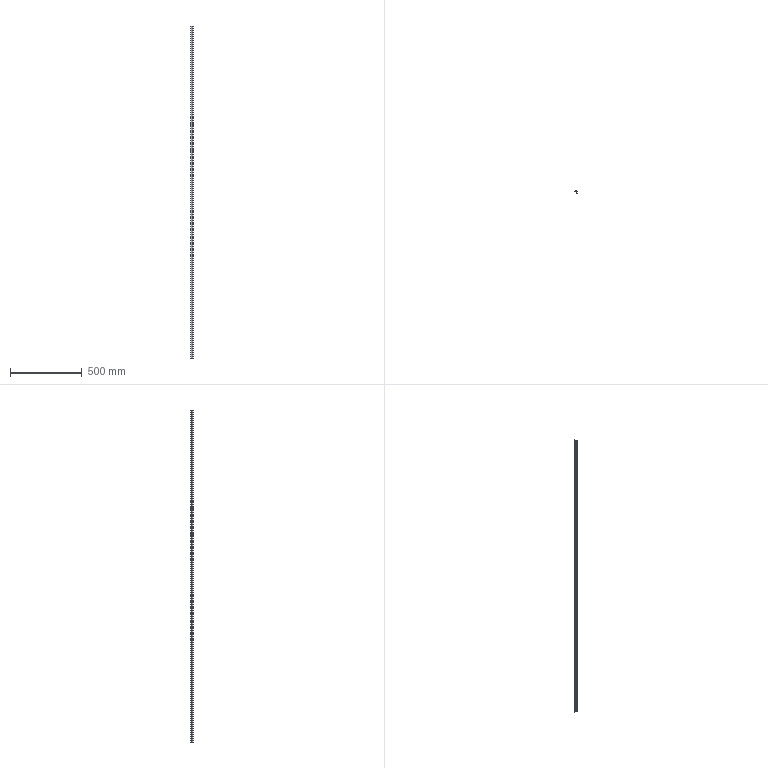Part | SolidWorks | features BaseBody 1, ICE 1, MoveFace 1 | 1 solid | 27 faces | box 14 x 20.3 x 2314 mm | volume 117819 mm3 | plane 20 | cylinder 7 | commonest cylinder face diameters 0.387 x2 0.8 x2 0.4 x1 20 x1 22 x1
STEP:
#1=CARTESIAN_POINT('',(-5.304,-0.625,200.));
#2=VERTEX_POINT('',#1);
#3=CARTESIAN_POINT('',(-5.449,-0.8125,200.));
#4=VERTEX_POINT('',#3);
#5=CARTESIAN_POINT('',(-5.255,-0.8125,200.));
#6=DIRECTION('',(0.,0.,1.));
#7=DIRECTION('',(-1.,0.,0.));
#8=AXIS2_PLACEMENT_3D('',#5,#6,#7);
#9=CIRCLE('',#8,0.1937);
#10=EDGE_CURVE('',#2,#4,#9,.T.);
#11=ORIENTED_EDGE('',*,*,#10,.T.);
#12=CARTESIAN_POINT('',(-5.449,-0.8125,-2114.));
#13=VERTEX_POINT('',#12);
#14=CARTESIAN_POINT('',(-5.449,-0.8125,230.));
#15=DIRECTION('',(0.,0.,-1.));
#16=VECTOR('',#15,1000.);
#17=LINE('',#14,#16);
#18=EDGE_CURVE('',#4,#13,#17,.T.);
#19=ORIENTED_EDGE('',*,*,#18,.T.);
#20=CARTESIAN_POINT('',(-5.304,-0.625,-2114.));
#21=VERTEX_POINT('',#20);
#22=CARTESIAN_POINT('',(-5.255,-0.8125,-2114.));
#23=DIRECTION('',(0.,0.,-1.));
#24=DIRECTION('',(1.,0.,0.));
#25=AXIS2_PLACEMENT_3D('',#22,#23,#24);
#26=CIRCLE('',#25,0.1937);
#27=EDGE_CURVE('',#13,#21,#26,.T.);
#28=ORIENTED_EDGE('',*,*,#27,.T.);
#29=CARTESIAN_POINT('',(-5.304,-0.625,230.));
#30=DIRECTION('',(0.,0.,-1.));
#31=VECTOR('',#30,1000.);
#32=LINE('',#29,#31);
#33=EDGE_CURVE('',#2,#21,#32,.T.);
#34=ORIENTED_EDGE('',*,*,#33,.F.);
#35=EDGE_LOOP('',(#11,#19,#28,#34));
#36=FACE_OUTER_BOUND('',#35,.T.);
#37=CARTESIAN_POINT('',(-5.255,-0.8125,230.));
#38=DIRECTION('',(0.,0.,-1.));
#39=DIRECTION('',(-1.,0.,0.));
#40=AXIS2_PLACEMENT_3D('',#37,#38,#39);
#41=CYLINDRICAL_SURFACE('',#40,0.1937);
#42=ADVANCED_FACE('',(#36),#41,.F.);
#43=CARTESIAN_POINT('',(5.,-1.,-2114.));
#44=VERTEX_POINT('',#43);
#45=CARTESIAN_POINT('',(5.,-14.3,-2114.));
#46=VERTEX_POINT('',#45);
#47=CARTESIAN_POINT('',(5.,29.623,-2114.));
#48=DIRECTION('',(0.,-1.,0.));
#49=VECTOR('',#48,1000.);
#50=LINE('',#47,#49);
#51=EDGE_CURVE('',#44,#46,#50,.T.);
#52=ORIENTED_EDGE('',*,*,#51,.F.);
#53=CARTESIAN_POINT('',(5.,-1.,200.));
#54=VERTEX_POINT('',#53);
#55=CARTESIAN_POINT('',(5.,-1.,230.));
#56=DIRECTION('',(0.,0.,-1.));
#57=VECTOR('',#56,1000.);
#58=LINE('',#55,#57);
#59=EDGE_CURVE('',#54,#44,#58,.T.);
#60=ORIENTED_EDGE('',*,*,#59,.F.);
#61=CARTESIAN_POINT('',(5.,-14.3,200.));
#62=VERTEX_POINT('',#61);
#63=CARTESIAN_POINT('',(5.,-14.3,200.));
#64=DIRECTION('',(0.,1.,0.));
#65=VECTOR('',#64,1000.);
#66=LINE('',#63,#65);
#67=EDGE_CURVE('',#62,#54,#66,.T.);
#68=ORIENTED_EDGE('',*,*,#67,.F.);
#69=CARTESIAN_POINT('',(5.,-14.3,230.));
#70=DIRECTION('',(0.,0.,1.));
#71=VECTOR('',#70,1000.);
#72=LINE('',#69,#71);
#73=EDGE_CURVE('',#46,#62,#72,.T.);
#74=ORIENTED_EDGE('',*,*,#73,.F.);
#75=EDGE_LOOP('',(#52,#60,#68,#74));
#76=FACE_OUTER_BOUND('',#75,.T.);
#77=CARTESIAN_POINT('',(5.,-14.3,230.));
#78=DIRECTION('',(-1.,0.,0.));
#79=DIRECTION('',(0.,0.,1.));
#80=AXIS2_PLACEMENT_3D('',#77,#78,#79);
#81=PLANE('',#80);
#82=ADVANCED_FACE('',(#76),#81,.F.);
#83=CARTESIAN_POINT('',(-9.,-2.,-2114.));
#84=VERTEX_POINT('',#83);
#85=CARTESIAN_POINT('',(-9.,-2.,200.));
#86=VERTEX_POINT('',#85);
#87=CARTESIAN_POINT('',(-9.,-2.,230.));
#88=DIRECTION('',(0.,0.,1.));
#89=VECTOR('',#88,1000.);
#90=LINE('',#87,#89);
#91=EDGE_CURVE('',#84,#86,#90,.T.);
#92=ORIENTED_EDGE('',*,*,#91,.F.);
#93=CARTESIAN_POINT('',(0.9,-2.,-2114.));
#94=VERTEX_POINT('',#93);
#95=CARTESIAN_POINT('',(5.,-2.,-2114.));
#96=DIRECTION('',(-1.,0.,0.));
#97=VECTOR('',#96,1000.);
#98=LINE('',#95,#97);
#99=EDGE_CURVE('',#94,#84,#98,.T.);
#100=ORIENTED_EDGE('',*,*,#99,.F.);
#101=CARTESIAN_POINT('',(0.9,-2.,200.));
#102=VERTEX_POINT('',#101);
#103=CARTESIAN_POINT('',(0.9,-2.,230.));
#104=DIRECTION('',(0.,0.,-1.));
#105=VECTOR('',#104,1000.);
#106=LINE('',#103,#105);
#107=EDGE_CURVE('',#102,#94,#106,.T.);
#108=ORIENTED_EDGE('',*,*,#107,.F.);
#109=CARTESIAN_POINT('',(5.,-2.,200.));
#110=DIRECTION('',(1.,0.,0.));
#111=VECTOR('',#110,1000.);
#112=LINE('',#109,#111);
#113=EDGE_CURVE('',#86,#102,#112,.T.);
#114=ORIENTED_EDGE('',*,*,#113,.F.);
#115=EDGE_LOOP('',(#92,#100,#108,#114));
#116=FACE_OUTER_BOUND('',#115,.T.);
#117=CARTESIAN_POINT('',(-9.,-2.,230.));
#118=DIRECTION('',(0.,1.,0.));
#119=DIRECTION('',(0.,0.,1.));
#120=AXIS2_PLACEMENT_3D('',#117,#118,#119);
#121=PLANE('',#120);
#122=ADVANCED_FACE('',(#116),#121,.F.);
#123=CARTESIAN_POINT('',(4.,-6.,200.));
#124=VERTEX_POINT('',#123);
#125=CARTESIAN_POINT('',(4.,-3.,200.));
#126=VERTEX_POINT('',#125);
#127=CARTESIAN_POINT('',(4.,29.623,200.));
#128=DIRECTION('',(0.,1.,0.));
#129=VECTOR('',#128,1000.);
#130=LINE('',#127,#129);
#131=EDGE_CURVE('',#124,#126,#130,.T.);
#132=ORIENTED_EDGE('',*,*,#131,.F.);
#133=CARTESIAN_POINT('',(1.,-6.,200.));
#134=VERTEX_POINT('',#133);
#135=CARTESIAN_POINT('',(5.,-6.,200.));
#136=DIRECTION('',(1.,0.,0.));
#137=VECTOR('',#136,1000.);
#138=LINE('',#135,#137);
#139=EDGE_CURVE('',#134,#124,#138,.T.);
#140=ORIENTED_EDGE('',*,*,#139,.F.);
#141=CARTESIAN_POINT('',(1.,-6.7,200.));
#142=VERTEX_POINT('',#141);
#143=CARTESIAN_POINT('',(1.,-6.,200.));
#144=DIRECTION('',(0.,-1.,0.));
#145=VECTOR('',#144,1000.);
#146=LINE('',#143,#145);
#147=EDGE_CURVE('',#134,#142,#146,.T.);
#148=ORIENTED_EDGE('',*,*,#147,.T.);
#149=CARTESIAN_POINT('',(-1.7,-6.7,200.));
#150=VERTEX_POINT('',#149);
#151=CARTESIAN_POINT('',(5.,-6.7,200.));
#152=DIRECTION('',(1.,0.,0.));
#153=VECTOR('',#152,1000.);
#154=LINE('',#151,#153);
#155=EDGE_CURVE('',#150,#142,#154,.T.);
#156=ORIENTED_EDGE('',*,*,#155,.F.);
#157=CARTESIAN_POINT('',(-1.7,-7.7,200.));
#158=VERTEX_POINT('',#157);
#159=CARTESIAN_POINT('',(-1.7,-6.7,200.));
#160=DIRECTION('',(0.,-1.,0.));
#161=VECTOR('',#160,1000.);
#162=LINE('',#159,#161);
#163=EDGE_CURVE('',#150,#158,#162,.T.);
#164=ORIENTED_EDGE('',*,*,#163,.T.);
#165=CARTESIAN_POINT('',(4.,-7.7,200.));
#166=VERTEX_POINT('',#165);
#167=CARTESIAN_POINT('',(5.,-7.7,200.));
#168=DIRECTION('',(-1.,0.,0.));
#169=VECTOR('',#168,1000.);
#170=LINE('',#167,#169);
#171=EDGE_CURVE('',#166,#158,#170,.T.);
#172=ORIENTED_EDGE('',*,*,#171,.F.);
#173=CARTESIAN_POINT('',(4.,-14.3,200.));
#174=VERTEX_POINT('',#173);
#175=CARTESIAN_POINT('',(4.,29.623,200.));
#176=DIRECTION('',(0.,1.,0.));
#177=VECTOR('',#176,1000.);
#178=LINE('',#175,#177);
#179=EDGE_CURVE('',#174,#166,#178,.T.);
#180=ORIENTED_EDGE('',*,*,#179,.F.);
#181=CARTESIAN_POINT('',(5.,-14.3,200.));
#182=DIRECTION('',(-1.,0.,0.));
#183=VECTOR('',#182,1000.);
#184=LINE('',#181,#183);
#185=EDGE_CURVE('',#62,#174,#184,.T.);
#186=ORIENTED_EDGE('',*,*,#185,.F.);
#187=ORIENTED_EDGE('',*,*,#67,.T.);
#188=CARTESIAN_POINT('',(-5.207,-1.,200.));
#189=VERTEX_POINT('',#188);
#190=CARTESIAN_POINT('',(5.,-1.,200.));
#191=DIRECTION('',(1.,0.,0.));
#192=VECTOR('',#191,1000.);
#193=LINE('',#190,#192);
#194=EDGE_CURVE('',#189,#54,#193,.T.);
#195=ORIENTED_EDGE('',*,*,#194,.F.);
#196=CARTESIAN_POINT('',(-5.255,-0.8125,200.));
#197=DIRECTION('',(0.,0.,1.));
#198=DIRECTION('',(-1.,0.,0.));
#199=AXIS2_PLACEMENT_3D('',#196,#197,#198);
#200=CIRCLE('',#199,0.1937);
#201=EDGE_CURVE('',#4,#189,#200,.T.);
#202=ORIENTED_EDGE('',*,*,#201,.F.);
#203=ORIENTED_EDGE('',*,*,#10,.F.);
#204=CARTESIAN_POINT('',(-1.368,3.063,200.));
#205=VERTEX_POINT('',#204);
#206=CARTESIAN_POINT('',(-10.628,9.,200.));
#207=DIRECTION('',(0.,0.,1.));
#208=DIRECTION('',(-1.,0.,0.));
#209=AXIS2_PLACEMENT_3D('',#206,#207,#208);
#210=CIRCLE('',#209,11.);
#211=EDGE_CURVE('',#2,#205,#210,.T.);
#212=ORIENTED_EDGE('',*,*,#211,.T.);
#213=CARTESIAN_POINT('',(-1.,2.955,200.));
#214=VERTEX_POINT('',#213);
#215=CARTESIAN_POINT('',(-1.2,2.955,200.));
#216=DIRECTION('',(0.,0.,1.));
#217=DIRECTION('',(-1.,0.,0.));
#218=AXIS2_PLACEMENT_3D('',#215,#216,#217);
#219=CIRCLE('',#218,0.2);
#220=EDGE_CURVE('',#214,#205,#219,.T.);
#221=ORIENTED_EDGE('',*,*,#220,.F.);
#222=CARTESIAN_POINT('',(-1.,1.5,200.));
#223=VERTEX_POINT('',#222);
#224=CARTESIAN_POINT('',(-1.,2.955,200.));
#225=DIRECTION('',(0.,1.,0.));
#226=VECTOR('',#225,1000.);
#227=LINE('',#224,#226);
#228=EDGE_CURVE('',#223,#214,#227,.T.);
#229=ORIENTED_EDGE('',*,*,#228,.F.);
#230=CARTESIAN_POINT('',(0.,1.5,200.));
#231=VERTEX_POINT('',#230);
#232=CARTESIAN_POINT('',(-1.,1.5,200.));
#233=DIRECTION('',(-1.,0.,0.));
#234=VECTOR('',#233,1000.);
#235=LINE('',#232,#234);
#236=EDGE_CURVE('',#231,#223,#235,.T.);
#237=ORIENTED_EDGE('',*,*,#236,.F.);
#238=CARTESIAN_POINT('',(0.,6.,200.));
#239=VERTEX_POINT('',#238);
#240=CARTESIAN_POINT('',(0.,1.5,200.));
#241=DIRECTION('',(0.,-1.,0.));
#242=VECTOR('',#241,1000.);
#243=LINE('',#240,#242);
#244=EDGE_CURVE('',#239,#231,#243,.T.);
#245=ORIENTED_EDGE('',*,*,#244,.F.);
#246=CARTESIAN_POINT('',(-0.8,6.,200.));
#247=VERTEX_POINT('',#246);
#248=CARTESIAN_POINT('',(0.,6.,200.));
#249=DIRECTION('',(1.,0.,0.));
#250=VECTOR('',#249,1000.);
#251=LINE('',#248,#250);
#252=EDGE_CURVE('',#247,#239,#251,.T.);
#253=ORIENTED_EDGE('',*,*,#252,.F.);
#254=CARTESIAN_POINT('',(-1.178,5.731,200.));
#255=VERTEX_POINT('',#254);
#256=CARTESIAN_POINT('',(-0.8,5.6,200.));
#257=DIRECTION('',(0.,0.,1.));
#258=DIRECTION('',(-1.,0.,0.));
#259=AXIS2_PLACEMENT_3D('',#256,#257,#258);
#260=CIRCLE('',#259,0.4);
#261=EDGE_CURVE('',#247,#255,#260,.T.);
#262=ORIENTED_EDGE('',*,*,#261,.T.);
#263=CARTESIAN_POINT('',(-8.678,-0.8077,200.));
#264=VERTEX_POINT('',#263);
#265=CARTESIAN_POINT('',(-10.628,9.,200.));
#266=DIRECTION('',(0.,0.,1.));
#267=DIRECTION('',(-1.,0.,0.));
#268=AXIS2_PLACEMENT_3D('',#265,#266,#267);
#269=CIRCLE('',#268,10.);
#270=EDGE_CURVE('',#264,#255,#269,.T.);
#271=ORIENTED_EDGE('',*,*,#270,.F.);
#272=CARTESIAN_POINT('',(-9.,-1.2,200.));
#273=VERTEX_POINT('',#272);
#274=CARTESIAN_POINT('',(-8.6,-1.2,200.));
#275=DIRECTION('',(0.,0.,1.));
#276=DIRECTION('',(-1.,0.,0.));
#277=AXIS2_PLACEMENT_3D('',#274,#275,#276);
#278=CIRCLE('',#277,0.4);
#279=EDGE_CURVE('',#264,#273,#278,.T.);
#280=ORIENTED_EDGE('',*,*,#279,.T.);
#281=CARTESIAN_POINT('',(-9.,8.,200.));
#282=DIRECTION('',(0.,-1.,0.));
#283=VECTOR('',#282,1000.);
#284=LINE('',#281,#283);
#285=EDGE_CURVE('',#273,#86,#284,.T.);
#286=ORIENTED_EDGE('',*,*,#285,.T.);
#287=ORIENTED_EDGE('',*,*,#113,.T.);
#288=CARTESIAN_POINT('',(0.9,-3.,200.));
#289=VERTEX_POINT('',#288);
#290=CARTESIAN_POINT('',(0.9,29.623,200.));
#291=DIRECTION('',(0.,1.,0.));
#292=VECTOR('',#291,1000.);
#293=LINE('',#290,#292);
#294=EDGE_CURVE('',#289,#102,#293,.T.);
#295=ORIENTED_EDGE('',*,*,#294,.F.);
#296=CARTESIAN_POINT('',(5.,-3.,200.));
#297=DIRECTION('',(-1.,0.,0.));
#298=VECTOR('',#297,1000.);
#299=LINE('',#296,#298);
#300=EDGE_CURVE('',#126,#289,#299,.T.);
#301=ORIENTED_EDGE('',*,*,#300,.F.);
#302=EDGE_LOOP('',(#132,#140,#148,#156,#164,#172,#180,#186,#187,#195,#202,#203,#212,#221,#229,#237,#245,#253,#262,#271,#280,#286,#287,#295,#301));
#303=FACE_OUTER_BOUND('',#302,.T.);
#304=CARTESIAN_POINT('',(5.,29.623,200.));
#305=DIRECTION('',(0.,0.,-1.));
#306=DIRECTION('',(-1.,0.,0.));
#307=AXIS2_PLACEMENT_3D('',#304,#305,#306);
#308=PLANE('',#307);
#309=ADVANCED_FACE('',(#303),#308,.F.);
#310=ORIENTED_EDGE('',*,*,#185,.T.);
#311=CARTESIAN_POINT('',(4.,-14.3,-2114.));
#312=VERTEX_POINT('',#311);
#313=CARTESIAN_POINT('',(4.,-14.3,230.));
#314=DIRECTION('',(0.,0.,1.));
#315=VECTOR('',#314,1000.);
#316=LINE('',#313,#315);
#317=EDGE_CURVE('',#312,#174,#316,.T.);
#318=ORIENTED_EDGE('',*,*,#317,.F.);
#319=CARTESIAN_POINT('',(5.,-14.3,-2114.));
#320=DIRECTION('',(-1.,0.,0.));
#321=VECTOR('',#320,1000.);
#322=LINE('',#319,#321);
#323=EDGE_CURVE('',#46,#312,#322,.T.);
#324=ORIENTED_EDGE('',*,*,#323,.F.);
#325=ORIENTED_EDGE('',*,*,#73,.T.);
#326=EDGE_LOOP('',(#310,#318,#324,#325));
#327=FACE_OUTER_BOUND('',#326,.T.);
#328=CARTESIAN_POINT('',(4.,-14.3,230.));
#329=DIRECTION('',(0.,1.,0.));
#330=DIRECTION('',(0.,0.,1.));
#331=AXIS2_PLACEMENT_3D('',#328,#329,#330);
#332=PLANE('',#331);
#333=ADVANCED_FACE('',(#327),#332,.F.);
#334=ORIENTED_EDGE('',*,*,#51,.T.);
#335=ORIENTED_EDGE('',*,*,#323,.T.);
#336=CARTESIAN_POINT('',(4.,-7.7,-2114.));
#337=VERTEX_POINT('',#336);
#338=CARTESIAN_POINT('',(4.,-7.7,-2114.));
#339=DIRECTION('',(0.,-1.,0.));
#340=VECTOR('',#339,1000.);
#341=LINE('',#338,#340);
#342=EDGE_CURVE('',#337,#312,#341,.T.);
#343=ORIENTED_EDGE('',*,*,#342,.F.);
#344=CARTESIAN_POINT('',(-1.7,-7.7,-2114.));
#345=VERTEX_POINT('',#344);
#346=CARTESIAN_POINT('',(-1.7,-7.7,-2114.));
#347=DIRECTION('',(1.,0.,0.));
#348=VECTOR('',#347,1000.);
#349=LINE('',#346,#348);
#350=EDGE_CURVE('',#345,#337,#349,.T.);
#351=ORIENTED_EDGE('',*,*,#350,.F.);
#352=CARTESIAN_POINT('',(-1.7,-6.7,-2114.));
#353=VERTEX_POINT('',#352);
#354=CARTESIAN_POINT('',(-1.7,29.623,-2114.));
#355=DIRECTION('',(0.,1.,0.));
#356=VECTOR('',#355,1000.);
#357=LINE('',#354,#356);
#358=EDGE_CURVE('',#345,#353,#357,.T.);
#359=ORIENTED_EDGE('',*,*,#358,.T.);
#360=CARTESIAN_POINT('',(1.,-6.7,-2114.));
#361=VERTEX_POINT('',#360);
#362=CARTESIAN_POINT('',(1.,-6.7,-2114.));
#363=DIRECTION('',(-1.,0.,0.));
#364=VECTOR('',#363,1000.);
#365=LINE('',#362,#364);
#366=EDGE_CURVE('',#361,#353,#365,.T.);
#367=ORIENTED_EDGE('',*,*,#366,.F.);
#368=CARTESIAN_POINT('',(1.,-6.,-2114.));
#369=VERTEX_POINT('',#368);
#370=CARTESIAN_POINT('',(1.,29.623,-2114.));
#371=DIRECTION('',(0.,1.,0.));
#372=VECTOR('',#371,1000.);
#373=LINE('',#370,#372);
#374=EDGE_CURVE('',#361,#369,#373,.T.);
#375=ORIENTED_EDGE('',*,*,#374,.T.);
#376=CARTESIAN_POINT('',(4.,-6.,-2114.));
#377=VERTEX_POINT('',#376);
#378=CARTESIAN_POINT('',(4.,-6.,-2114.));
#379=DIRECTION('',(-1.,0.,0.));
#380=VECTOR('',#379,1000.);
#381=LINE('',#378,#380);
#382=EDGE_CURVE('',#377,#369,#381,.T.);
#383=ORIENTED_EDGE('',*,*,#382,.F.);
#384=CARTESIAN_POINT('',(4.,-3.,-2114.));
#385=VERTEX_POINT('',#384);
#386=CARTESIAN_POINT('',(4.,-3.,-2114.));
#387=DIRECTION('',(0.,-1.,0.));
#388=VECTOR('',#387,1000.);
#389=LINE('',#386,#388);
#390=EDGE_CURVE('',#385,#377,#389,.T.);
#391=ORIENTED_EDGE('',*,*,#390,.F.);
#392=CARTESIAN_POINT('',(0.9,-3.,-2114.));
#393=VERTEX_POINT('',#392);
#394=CARTESIAN_POINT('',(0.9,-3.,-2114.));
#395=DIRECTION('',(1.,0.,0.));
#396=VECTOR('',#395,1000.);
#397=LINE('',#394,#396);
#398=EDGE_CURVE('',#393,#385,#397,.T.);
#399=ORIENTED_EDGE('',*,*,#398,.F.);
#400=CARTESIAN_POINT('',(0.9,-2.,-2114.));
#401=DIRECTION('',(0.,-1.,0.));
#402=VECTOR('',#401,1000.);
#403=LINE('',#400,#402);
#404=EDGE_CURVE('',#94,#393,#403,.T.);
#405=ORIENTED_EDGE('',*,*,#404,.F.);
#406=ORIENTED_EDGE('',*,*,#99,.T.);
#407=CARTESIAN_POINT('',(-9.,-1.2,-2114.));
#408=VERTEX_POINT('',#407);
#409=CARTESIAN_POINT('',(-9.,-1.2,-2114.));
#410=DIRECTION('',(0.,-1.,0.));
#411=VECTOR('',#410,1000.);
#412=LINE('',#409,#411);
#413=EDGE_CURVE('',#408,#84,#412,.T.);
#414=ORIENTED_EDGE('',*,*,#413,.F.);
#415=CARTESIAN_POINT('',(-8.678,-0.8077,-2114.));
#416=VERTEX_POINT('',#415);
#417=CARTESIAN_POINT('',(-8.6,-1.2,-2114.));
#418=DIRECTION('',(0.,0.,-1.));
#419=DIRECTION('',(1.,0.,0.));
#420=AXIS2_PLACEMENT_3D('',#417,#418,#419);
#421=CIRCLE('',#420,0.4);
#422=EDGE_CURVE('',#408,#416,#421,.T.);
#423=ORIENTED_EDGE('',*,*,#422,.T.);
#424=CARTESIAN_POINT('',(-1.178,5.731,-2114.));
#425=VERTEX_POINT('',#424);
#426=CARTESIAN_POINT('',(-10.628,9.,-2114.));
#427=DIRECTION('',(0.,0.,-1.));
#428=DIRECTION('',(1.,0.,0.));
#429=AXIS2_PLACEMENT_3D('',#426,#427,#428);
#430=CIRCLE('',#429,10.);
#431=EDGE_CURVE('',#425,#416,#430,.T.);
#432=ORIENTED_EDGE('',*,*,#431,.F.);
#433=CARTESIAN_POINT('',(-0.8,6.,-2114.));
#434=VERTEX_POINT('',#433);
#435=CARTESIAN_POINT('',(-0.8,5.6,-2114.));
#436=DIRECTION('',(0.,0.,-1.));
#437=DIRECTION('',(1.,0.,0.));
#438=AXIS2_PLACEMENT_3D('',#435,#436,#437);
#439=CIRCLE('',#438,0.4);
#440=EDGE_CURVE('',#425,#434,#439,.T.);
#441=ORIENTED_EDGE('',*,*,#440,.T.);
#442=CARTESIAN_POINT('',(0.,6.,-2114.));
#443=VERTEX_POINT('',#442);
#444=CARTESIAN_POINT('',(0.,6.,-2114.));
#445=DIRECTION('',(-1.,0.,0.));
#446=VECTOR('',#445,1000.);
#447=LINE('',#444,#446);
#448=EDGE_CURVE('',#443,#434,#447,.T.);
#449=ORIENTED_EDGE('',*,*,#448,.F.);
#450=CARTESIAN_POINT('',(0.,1.5,-2114.));
#451=VERTEX_POINT('',#450);
#452=CARTESIAN_POINT('',(0.,1.5,-2114.));
#453=DIRECTION('',(0.,1.,0.));
#454=VECTOR('',#453,1000.);
#455=LINE('',#452,#454);
#456=EDGE_CURVE('',#451,#443,#455,.T.);
#457=ORIENTED_EDGE('',*,*,#456,.F.);
#458=CARTESIAN_POINT('',(-1.,1.5,-2114.));
#459=VERTEX_POINT('',#458);
#460=CARTESIAN_POINT('',(-1.,1.5,-2114.));
#461=DIRECTION('',(1.,0.,0.));
#462=VECTOR('',#461,1000.);
#463=LINE('',#460,#462);
#464=EDGE_CURVE('',#459,#451,#463,.T.);
#465=ORIENTED_EDGE('',*,*,#464,.F.);
#466=CARTESIAN_POINT('',(-1.,2.955,-2114.));
#467=VERTEX_POINT('',#466);
#468=CARTESIAN_POINT('',(-1.,2.955,-2114.));
#469=DIRECTION('',(0.,-1.,0.));
#470=VECTOR('',#469,1000.);
#471=LINE('',#468,#470);
#472=EDGE_CURVE('',#467,#459,#471,.T.);
#473=ORIENTED_EDGE('',*,*,#472,.F.);
#474=CARTESIAN_POINT('',(-1.368,3.063,-2114.));
#475=VERTEX_POINT('',#474);
#476=CARTESIAN_POINT('',(-1.2,2.955,-2114.));
#477=DIRECTION('',(0.,0.,-1.));
#478=DIRECTION('',(1.,0.,0.));
#479=AXIS2_PLACEMENT_3D('',#476,#477,#478);
#480=CIRCLE('',#479,0.2);
#481=EDGE_CURVE('',#475,#467,#480,.T.);
#482=ORIENTED_EDGE('',*,*,#481,.F.);
#483=CARTESIAN_POINT('',(-10.628,9.,-2114.));
#484=DIRECTION('',(0.,0.,-1.));
#485=DIRECTION('',(1.,0.,0.));
#486=AXIS2_PLACEMENT_3D('',#483,#484,#485);
#487=CIRCLE('',#486,11.);
#488=EDGE_CURVE('',#475,#21,#487,.T.);
#489=ORIENTED_EDGE('',*,*,#488,.T.);
#490=ORIENTED_EDGE('',*,*,#27,.F.);
#491=CARTESIAN_POINT('',(-5.207,-1.,-2114.));
#492=VERTEX_POINT('',#491);
#493=CARTESIAN_POINT('',(-5.255,-0.8125,-2114.));
#494=DIRECTION('',(0.,0.,-1.));
#495=DIRECTION('',(1.,0.,0.));
#496=AXIS2_PLACEMENT_3D('',#493,#494,#495);
#497=CIRCLE('',#496,0.1937);
#498=EDGE_CURVE('',#492,#13,#497,.T.);
#499=ORIENTED_EDGE('',*,*,#498,.F.);
#500=CARTESIAN_POINT('',(5.,-1.,-2114.));
#501=DIRECTION('',(-1.,0.,0.));
#502=VECTOR('',#501,1000.);
#503=LINE('',#500,#502);
#504=EDGE_CURVE('',#44,#492,#503,.T.);
#505=ORIENTED_EDGE('',*,*,#504,.F.);
#506=EDGE_LOOP('',(#334,#335,#343,#351,#359,#367,#375,#383,#391,#399,#405,#406,#414,#423,#432,#441,#449,#457,#465,#473,#482,#489,#490,#499,#505));
#507=FACE_OUTER_BOUND('',#506,.T.);
#508=CARTESIAN_POINT('',(5.,29.623,-2114.));
#509=DIRECTION('',(0.,0.,1.));
#510=DIRECTION('',(1.,0.,0.));
#511=AXIS2_PLACEMENT_3D('',#508,#509,#510);
#512=PLANE('',#511);
#513=ADVANCED_FACE('',(#507),#512,.F.);
#514=ORIENTED_EDGE('',*,*,#59,.T.);
#515=ORIENTED_EDGE('',*,*,#504,.T.);
#516=CARTESIAN_POINT('',(-5.207,-1.,230.));
#517=DIRECTION('',(0.,0.,-1.));
#518=VECTOR('',#517,1000.);
#519=LINE('',#516,#518);
#520=EDGE_CURVE('',#189,#492,#519,.T.);
#521=ORIENTED_EDGE('',*,*,#520,.F.);
#522=ORIENTED_EDGE('',*,*,#194,.T.);
#523=EDGE_LOOP('',(#514,#515,#521,#522));
#524=FACE_OUTER_BOUND('',#523,.T.);
#525=CARTESIAN_POINT('',(5.,-1.,230.));
#526=DIRECTION('',(0.,-1.,0.));
#527=DIRECTION('',(0.,0.,-1.));
#528=AXIS2_PLACEMENT_3D('',#525,#526,#527);
#529=PLANE('',#528);
#530=ADVANCED_FACE('',(#524),#529,.F.);
#531=CARTESIAN_POINT('',(-9.,-1.2,230.));
#532=DIRECTION('',(0.,0.,1.));
#533=VECTOR('',#532,1000.);
#534=LINE('',#531,#533);
#535=EDGE_CURVE('',#408,#273,#534,.T.);
#536=ORIENTED_EDGE('',*,*,#535,.F.);
#537=ORIENTED_EDGE('',*,*,#413,.T.);
#538=ORIENTED_EDGE('',*,*,#91,.T.);
#539=ORIENTED_EDGE('',*,*,#285,.F.);
#540=EDGE_LOOP('',(#536,#537,#538,#539));
#541=FACE_OUTER_BOUND('',#540,.T.);
#542=CARTESIAN_POINT('',(-9.,-1.2,230.));
#543=DIRECTION('',(1.,0.,0.));
#544=DIRECTION('',(0.,0.,-1.));
#545=AXIS2_PLACEMENT_3D('',#542,#543,#544);
#546=PLANE('',#545);
#547=ADVANCED_FACE('',(#541),#546,.F.);
#548=ORIENTED_EDGE('',*,*,#294,.T.);
#549=ORIENTED_EDGE('',*,*,#107,.T.);
#550=ORIENTED_EDGE('',*,*,#404,.T.);
#551=CARTESIAN_POINT('',(0.9,-3.,230.));
#552=DIRECTION('',(0.,0.,-1.));
#553=VECTOR('',#552,1000.);
#554=LINE('',#551,#553);
#555=EDGE_CURVE('',#289,#393,#554,.T.);
#556=ORIENTED_EDGE('',*,*,#555,.F.);
#557=EDGE_LOOP('',(#548,#549,#550,#556));
#558=FACE_OUTER_BOUND('',#557,.T.);
#559=CARTESIAN_POINT('',(0.9,-2.,230.));
#560=DIRECTION('',(1.,0.,0.));
#561=DIRECTION('',(0.,0.,-1.));
#562=AXIS2_PLACEMENT_3D('',#559,#560,#561);
#563=PLANE('',#562);
#564=ADVANCED_FACE('',(#558),#563,.F.);
#565=ORIENTED_EDGE('',*,*,#300,.T.);
#566=ORIENTED_EDGE('',*,*,#555,.T.);
#567=ORIENTED_EDGE('',*,*,#398,.T.);
#568=CARTESIAN_POINT('',(4.,-3.,230.));
#569=DIRECTION('',(0.,0.,-1.));
#570=VECTOR('',#569,1000.);
#571=LINE('',#568,#570);
#572=EDGE_CURVE('',#126,#385,#571,.T.);
#573=ORIENTED_EDGE('',*,*,#572,.F.);
#574=EDGE_LOOP('',(#565,#566,#567,#573));
#575=FACE_OUTER_BOUND('',#574,.T.);
#576=CARTESIAN_POINT('',(0.9,-3.,230.));
#577=DIRECTION('',(0.,1.,0.));
#578=DIRECTION('',(0.,0.,1.));
#579=AXIS2_PLACEMENT_3D('',#576,#577,#578);
#580=PLANE('',#579);
#581=ADVANCED_FACE('',(#575),#580,.F.);
#582=ORIENTED_EDGE('',*,*,#131,.T.);
#583=ORIENTED_EDGE('',*,*,#572,.T.);
#584=ORIENTED_EDGE('',*,*,#390,.T.);
#585=CARTESIAN_POINT('',(4.,-6.,230.));
#586=DIRECTION('',(0.,0.,-1.));
#587=VECTOR('',#586,1000.);
#588=LINE('',#585,#587);
#589=EDGE_CURVE('',#124,#377,#588,.T.);
#590=ORIENTED_EDGE('',*,*,#589,.F.);
#591=EDGE_LOOP('',(#582,#583,#584,#590));
#592=FACE_OUTER_BOUND('',#591,.T.);
#593=CARTESIAN_POINT('',(4.,-3.,230.));
#594=DIRECTION('',(1.,0.,0.));
#595=DIRECTION('',(0.,0.,-1.));
#596=AXIS2_PLACEMENT_3D('',#593,#594,#595);
#597=PLANE('',#596);
#598=ADVANCED_FACE('',(#592),#597,.F.);
#599=ORIENTED_EDGE('',*,*,#139,.T.);
#600=ORIENTED_EDGE('',*,*,#589,.T.);
#601=ORIENTED_EDGE('',*,*,#382,.T.);
#602=CARTESIAN_POINT('',(1.,-6.,230.));
#603=DIRECTION('',(0.,0.,-1.));
#604=VECTOR('',#603,1000.);
#605=LINE('',#602,#604);
#606=EDGE_CURVE('',#134,#369,#605,.T.);
#607=ORIENTED_EDGE('',*,*,#606,.F.);
#608=EDGE_LOOP('',(#599,#600,#601,#607));
#609=FACE_OUTER_BOUND('',#608,.T.);
#610=CARTESIAN_POINT('',(4.,-6.,230.));
#611=DIRECTION('',(0.,-1.,0.));
#612=DIRECTION('',(0.,0.,-1.));
#613=AXIS2_PLACEMENT_3D('',#610,#611,#612);
#614=PLANE('',#613);
#615=ADVANCED_FACE('',(#609),#614,.F.);
#616=ORIENTED_EDGE('',*,*,#155,.T.);
#617=CARTESIAN_POINT('',(1.,-6.7,230.));
#618=DIRECTION('',(0.,0.,1.));
#619=VECTOR('',#618,1000.);
#620=LINE('',#617,#619);
#621=EDGE_CURVE('',#361,#142,#620,.T.);
#622=ORIENTED_EDGE('',*,*,#621,.F.);
#623=ORIENTED_EDGE('',*,*,#366,.T.);
#624=CARTESIAN_POINT('',(-1.7,-6.7,230.));
#625=DIRECTION('',(0.,0.,-1.));
#626=VECTOR('',#625,1000.);
#627=LINE('',#624,#626);
#628=EDGE_CURVE('',#150,#353,#627,.T.);
#629=ORIENTED_EDGE('',*,*,#628,.F.);
#630=EDGE_LOOP('',(#616,#622,#623,#629));
#631=FACE_OUTER_BOUND('',#630,.T.);
#632=CARTESIAN_POINT('',(1.,-6.7,230.));
#633=DIRECTION('',(0.,-1.,0.));
#634=DIRECTION('',(0.,0.,-1.));
#635=AXIS2_PLACEMENT_3D('',#632,#633,#634);
#636=PLANE('',#635);
#637=ADVANCED_FACE('',(#631),#636,.F.);
#638=ORIENTED_EDGE('',*,*,#171,.T.);
#639=CARTESIAN_POINT('',(-1.7,-7.7,230.));
#640=DIRECTION('',(0.,0.,1.));
#641=VECTOR('',#640,1000.);
#642=LINE('',#639,#641);
#643=EDGE_CURVE('',#345,#158,#642,.T.);
#644=ORIENTED_EDGE('',*,*,#643,.F.);
#645=ORIENTED_EDGE('',*,*,#350,.T.);
#646=CARTESIAN_POINT('',(4.,-7.7,230.));
#647=DIRECTION('',(0.,0.,-1.));
#648=VECTOR('',#647,1000.);
#649=LINE('',#646,#648);
#650=EDGE_CURVE('',#166,#337,#649,.T.);
#651=ORIENTED_EDGE('',*,*,#650,.F.);
#652=EDGE_LOOP('',(#638,#644,#645,#651));
#653=FACE_OUTER_BOUND('',#652,.T.);
#654=CARTESIAN_POINT('',(-1.7,-7.7,230.));
#655=DIRECTION('',(0.,1.,0.));
#656=DIRECTION('',(0.,0.,1.));
#657=AXIS2_PLACEMENT_3D('',#654,#655,#656);
#658=PLANE('',#657);
#659=ADVANCED_FACE('',(#653),#658,.F.);
#660=ORIENTED_EDGE('',*,*,#179,.T.);
#661=ORIENTED_EDGE('',*,*,#650,.T.);
#662=ORIENTED_EDGE('',*,*,#342,.T.);
#663=ORIENTED_EDGE('',*,*,#317,.T.);
#664=EDGE_LOOP('',(#660,#661,#662,#663));
#665=FACE_OUTER_BOUND('',#664,.T.);
#666=CARTESIAN_POINT('',(4.,-7.7,230.));
#667=DIRECTION('',(1.,0.,0.));
#668=DIRECTION('',(0.,0.,-1.));
#669=AXIS2_PLACEMENT_3D('',#666,#667,#668);
#670=PLANE('',#669);
#671=ADVANCED_FACE('',(#665),#670,.F.);
#672=ORIENTED_EDGE('',*,*,#18,.F.);
#673=ORIENTED_EDGE('',*,*,#201,.T.);
#674=ORIENTED_EDGE('',*,*,#520,.T.);
#675=ORIENTED_EDGE('',*,*,#498,.T.);
#676=EDGE_LOOP('',(#672,#673,#674,#675));
#677=FACE_OUTER_BOUND('',#676,.T.);
#678=CARTESIAN_POINT('',(-5.255,-0.8125,230.));
#679=DIRECTION('',(0.,0.,-1.));
#680=DIRECTION('',(-1.,0.,0.));
#681=AXIS2_PLACEMENT_3D('',#678,#679,#680);
#682=CYLINDRICAL_SURFACE('',#681,0.1937);
#683=ADVANCED_FACE('',(#677),#682,.F.);
#684=CARTESIAN_POINT('',(-1.,2.955,230.));
#685=DIRECTION('',(0.,0.,1.));
#686=VECTOR('',#685,1000.);
#687=LINE('',#684,#686);
#688=EDGE_CURVE('',#467,#214,#687,.T.);
#689=ORIENTED_EDGE('',*,*,#688,.F.);
#690=ORIENTED_EDGE('',*,*,#472,.T.);
#691=CARTESIAN_POINT('',(-1.,1.5,230.));
#692=DIRECTION('',(0.,0.,-1.));
#693=VECTOR('',#692,1000.);
#694=LINE('',#691,#693);
#695=EDGE_CURVE('',#223,#459,#694,.T.);
#696=ORIENTED_EDGE('',*,*,#695,.F.);
#697=ORIENTED_EDGE('',*,*,#228,.T.);
#698=EDGE_LOOP('',(#689,#690,#696,#697));
#699=FACE_OUTER_BOUND('',#698,.T.);
#700=CARTESIAN_POINT('',(-1.,2.955,230.));
#701=DIRECTION('',(1.,0.,0.));
#702=DIRECTION('',(0.,0.,-1.));
#703=AXIS2_PLACEMENT_3D('',#700,#701,#702);
#704=PLANE('',#703);
#705=ADVANCED_FACE('',(#699),#704,.F.);
#706=ORIENTED_EDGE('',*,*,#488,.F.);
#707=CARTESIAN_POINT('',(-1.368,3.063,230.));
#708=DIRECTION('',(0.,0.,1.));
#709=VECTOR('',#708,1000.);
#710=LINE('',#707,#709);
#711=EDGE_CURVE('',#475,#205,#710,.T.);
#712=ORIENTED_EDGE('',*,*,#711,.T.);
#713=ORIENTED_EDGE('',*,*,#211,.F.);
#714=ORIENTED_EDGE('',*,*,#33,.T.);
#715=EDGE_LOOP('',(#706,#712,#713,#714));
#716=FACE_OUTER_BOUND('',#715,.T.);
#717=CARTESIAN_POINT('',(-10.628,9.,230.));
#718=DIRECTION('',(0.,0.,-1.));
#719=DIRECTION('',(-1.,0.,0.));
#720=AXIS2_PLACEMENT_3D('',#717,#718,#719);
#721=CYLINDRICAL_SURFACE('',#720,11.);
#722=ADVANCED_FACE('',(#716),#721,.T.);
#723=CARTESIAN_POINT('',(-1.178,5.731,230.));
#724=DIRECTION('',(0.,0.,1.));
#725=VECTOR('',#724,1000.);
#726=LINE('',#723,#725);
#727=EDGE_CURVE('',#425,#255,#726,.T.);
#728=ORIENTED_EDGE('',*,*,#727,.F.);
#729=ORIENTED_EDGE('',*,*,#431,.T.);
#730=CARTESIAN_POINT('',(-8.678,-0.8077,230.));
#731=DIRECTION('',(0.,0.,-1.));
#732=VECTOR('',#731,1000.);
#733=LINE('',#730,#732);
#734=EDGE_CURVE('',#264,#416,#733,.T.);
#735=ORIENTED_EDGE('',*,*,#734,.F.);
#736=ORIENTED_EDGE('',*,*,#270,.T.);
#737=EDGE_LOOP('',(#728,#729,#735,#736));
#738=FACE_OUTER_BOUND('',#737,.T.);
#739=CARTESIAN_POINT('',(-10.628,9.,230.));
#740=DIRECTION('',(0.,0.,-1.));
#741=DIRECTION('',(-1.,0.,0.));
#742=AXIS2_PLACEMENT_3D('',#739,#740,#741);
#743=CYLINDRICAL_SURFACE('',#742,10.);
#744=ADVANCED_FACE('',(#738),#743,.F.);
#745=CARTESIAN_POINT('',(0.,1.5,230.));
#746=DIRECTION('',(0.,0.,1.));
#747=VECTOR('',#746,1000.);
#748=LINE('',#745,#747);
#749=EDGE_CURVE('',#451,#231,#748,.T.);
#750=ORIENTED_EDGE('',*,*,#749,.F.);
#751=ORIENTED_EDGE('',*,*,#456,.T.);
#752=CARTESIAN_POINT('',(0.,6.,230.));
#753=DIRECTION('',(0.,0.,-1.));
#754=VECTOR('',#753,1000.);
#755=LINE('',#752,#754);
#756=EDGE_CURVE('',#239,#443,#755,.T.);
#757=ORIENTED_EDGE('',*,*,#756,.F.);
#758=ORIENTED_EDGE('',*,*,#244,.T.);
#759=EDGE_LOOP('',(#750,#751,#757,#758));
#760=FACE_OUTER_BOUND('',#759,.T.);
#761=CARTESIAN_POINT('',(0.,1.5,230.));
#762=DIRECTION('',(-1.,0.,0.));
#763=DIRECTION('',(0.,0.,1.));
#764=AXIS2_PLACEMENT_3D('',#761,#762,#763);
#765=PLANE('',#764);
#766=ADVANCED_FACE('',(#760),#765,.F.);
#767=ORIENTED_EDGE('',*,*,#422,.F.);
#768=ORIENTED_EDGE('',*,*,#535,.T.);
#769=ORIENTED_EDGE('',*,*,#279,.F.);
#770=ORIENTED_EDGE('',*,*,#734,.T.);
#771=EDGE_LOOP('',(#767,#768,#769,#770));
#772=FACE_OUTER_BOUND('',#771,.T.);
#773=CARTESIAN_POINT('',(-8.6,-1.2,230.));
#774=DIRECTION('',(0.,0.,-1.));
#775=DIRECTION('',(-1.,0.,0.));
#776=AXIS2_PLACEMENT_3D('',#773,#774,#775);
#777=CYLINDRICAL_SURFACE('',#776,0.4);
#778=ADVANCED_FACE('',(#772),#777,.T.);
#779=ORIENTED_EDGE('',*,*,#147,.F.);
#780=ORIENTED_EDGE('',*,*,#606,.T.);
#781=ORIENTED_EDGE('',*,*,#374,.F.);
#782=ORIENTED_EDGE('',*,*,#621,.T.);
#783=EDGE_LOOP('',(#779,#780,#781,#782));
#784=FACE_OUTER_BOUND('',#783,.T.);
#785=CARTESIAN_POINT('',(1.,-6.,230.));
#786=DIRECTION('',(1.,0.,0.));
#787=DIRECTION('',(0.,0.,-1.));
#788=AXIS2_PLACEMENT_3D('',#785,#786,#787);
#789=PLANE('',#788);
#790=ADVANCED_FACE('',(#784),#789,.F.);
#791=ORIENTED_EDGE('',*,*,#163,.F.);
#792=ORIENTED_EDGE('',*,*,#628,.T.);
#793=ORIENTED_EDGE('',*,*,#358,.F.);
#794=ORIENTED_EDGE('',*,*,#643,.T.);
#795=EDGE_LOOP('',(#791,#792,#793,#794));
#796=FACE_OUTER_BOUND('',#795,.T.);
#797=CARTESIAN_POINT('',(-1.7,-6.7,230.));
#798=DIRECTION('',(1.,0.,0.));
#799=DIRECTION('',(0.,0.,-1.));
#800=AXIS2_PLACEMENT_3D('',#797,#798,#799);
#801=PLANE('',#800);
#802=ADVANCED_FACE('',(#796),#801,.F.);
#803=ORIENTED_EDGE('',*,*,#711,.F.);
#804=ORIENTED_EDGE('',*,*,#481,.T.);
#805=ORIENTED_EDGE('',*,*,#688,.T.);
#806=ORIENTED_EDGE('',*,*,#220,.T.);
#807=EDGE_LOOP('',(#803,#804,#805,#806));
#808=FACE_OUTER_BOUND('',#807,.T.);
#809=CARTESIAN_POINT('',(-1.2,2.955,230.));
#810=DIRECTION('',(0.,0.,-1.));
#811=DIRECTION('',(-1.,0.,0.));
#812=AXIS2_PLACEMENT_3D('',#809,#810,#811);
#813=CYLINDRICAL_SURFACE('',#812,0.2);
#814=ADVANCED_FACE('',(#808),#813,.F.);
#815=ORIENTED_EDGE('',*,*,#695,.T.);
#816=ORIENTED_EDGE('',*,*,#464,.T.);
#817=ORIENTED_EDGE('',*,*,#749,.T.);
#818=ORIENTED_EDGE('',*,*,#236,.T.);
#819=EDGE_LOOP('',(#815,#816,#817,#818));
#820=FACE_OUTER_BOUND('',#819,.T.);
#821=CARTESIAN_POINT('',(-1.,1.5,230.));
#822=DIRECTION('',(0.,1.,0.));
#823=DIRECTION('',(0.,0.,1.));
#824=AXIS2_PLACEMENT_3D('',#821,#822,#823);
#825=PLANE('',#824);
#826=ADVANCED_FACE('',(#820),#825,.F.);
#827=ORIENTED_EDGE('',*,*,#440,.F.);
#828=ORIENTED_EDGE('',*,*,#727,.T.);
#829=ORIENTED_EDGE('',*,*,#261,.F.);
#830=CARTESIAN_POINT('',(-0.8,6.,230.));
#831=DIRECTION('',(0.,0.,-1.));
#832=VECTOR('',#831,1000.);
#833=LINE('',#830,#832);
#834=EDGE_CURVE('',#247,#434,#833,.T.);
#835=ORIENTED_EDGE('',*,*,#834,.T.);
#836=EDGE_LOOP('',(#827,#828,#829,#835));
#837=FACE_OUTER_BOUND('',#836,.T.);
#838=CARTESIAN_POINT('',(-0.8,5.6,230.));
#839=DIRECTION('',(0.,0.,-1.));
#840=DIRECTION('',(-1.,0.,0.));
#841=AXIS2_PLACEMENT_3D('',#838,#839,#840);
#842=CYLINDRICAL_SURFACE('',#841,0.4);
#843=ADVANCED_FACE('',(#837),#842,.T.);
#844=ORIENTED_EDGE('',*,*,#756,.T.);
#845=ORIENTED_EDGE('',*,*,#448,.T.);
#846=ORIENTED_EDGE('',*,*,#834,.F.);
#847=ORIENTED_EDGE('',*,*,#252,.T.);
#848=EDGE_LOOP('',(#844,#845,#846,#847));
#849=FACE_OUTER_BOUND('',#848,.T.);
#850=CARTESIAN_POINT('',(0.,6.,230.));
#851=DIRECTION('',(0.,-1.,0.));
#852=DIRECTION('',(0.,0.,-1.));
#853=AXIS2_PLACEMENT_3D('',#850,#851,#852);
#854=PLANE('',#853);
#855=ADVANCED_FACE('',(#849),#854,.F.);
#856=CLOSED_SHELL('',(#42,#82,#122,#309,#333,#513,#530,#547,#564,#581,#598,#615,#637,#659,#671,#683,#705,#722,#744,#766,#778,#790,#802,#814,#826,#843,#855));
#857=MANIFOLD_SOLID_BREP('',#856);
#858=CARTESIAN_POINT('',(0.,0.,0.));
#859=DIRECTION('',(0.,0.,1.));
#860=DIRECTION('',(1.,0.,0.));
#861=AXIS2_PLACEMENT_3D('',#858,#859,#860);
#862=(LENGTH_UNIT()NAMED_UNIT(*)SI_UNIT(.MILLI.,.METRE.));
#863=UNCERTAINTY_MEASURE_WITH_UNIT(LENGTH_MEASURE(0.00001),#862,'','');
#864=(NAMED_UNIT(*)PLANE_ANGLE_UNIT()SI_UNIT($,.RADIAN.));
#865=(NAMED_UNIT(*)SI_UNIT($,.STERADIAN.)SOLID_ANGLE_UNIT());
#866=(GEOMETRIC_REPRESENTATION_CONTEXT(3)GLOBAL_UNCERTAINTY_ASSIGNED_CONTEXT((#863))GLOBAL_UNIT_ASSIGNED_CONTEXT((#862,#864,#865))REPRESENTATION_CONTEXT('',''));
#867=ADVANCED_BREP_SHAPE_REPRESENTATION('',(#857,#861),#866);